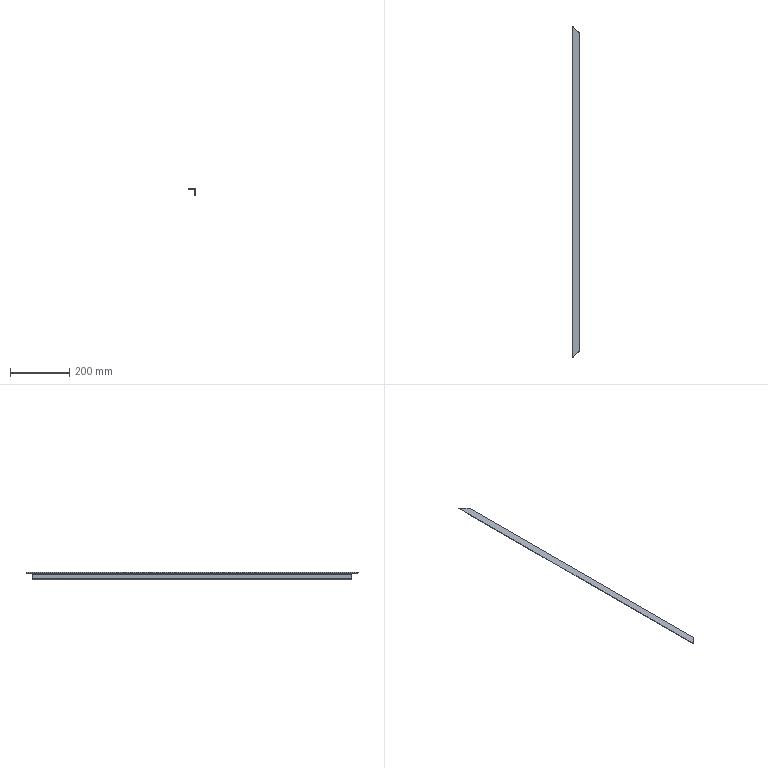Part | STEP file | Guide wheel mechanism revised.sldasm-Part-16 | 1 solid | 9 faces | box 25 x 1120 x 25 mm | volume 195019 mm3 | plane 6 | cylinder 3 | commonest cylinder face diameters 8 x2 7 x1
STEP:
#1=CARTESIAN_POINT('',(-430.,1915.,-505.));
#2=VERTEX_POINT('',#1);
#3=CARTESIAN_POINT('',(-405.,1890.,-505.));
#4=VERTEX_POINT('',#3);
#5=CARTESIAN_POINT('',(117.5,1367.5,-505.));
#6=DIRECTION('',(0.7071,-0.7071,0.));
#7=VECTOR('',#6,1000.);
#8=LINE('',#5,#7);
#9=EDGE_CURVE('',#2,#4,#8,.T.);
#10=ORIENTED_EDGE('',*,*,#9,.F.);
#11=CARTESIAN_POINT('',(-430.,795.,-505.));
#12=VERTEX_POINT('',#11);
#13=CARTESIAN_POINT('',(-430.,820.,-505.));
#14=DIRECTION('',(0.,1.,0.));
#15=VECTOR('',#14,1000.);
#16=LINE('',#13,#15);
#17=EDGE_CURVE('',#12,#2,#16,.T.);
#18=ORIENTED_EDGE('',*,*,#17,.F.);
#19=CARTESIAN_POINT('',(-405.,820.,-505.));
#20=VERTEX_POINT('',#19);
#21=CARTESIAN_POINT('',(-417.5,807.5,-505.));
#22=DIRECTION('',(-0.7071,-0.7071,0.));
#23=VECTOR('',#22,1000.);
#24=LINE('',#21,#23);
#25=EDGE_CURVE('',#20,#12,#24,.T.);
#26=ORIENTED_EDGE('',*,*,#25,.F.);
#27=CARTESIAN_POINT('',(-405.,820.,-505.));
#28=DIRECTION('',(0.,1.,0.));
#29=VECTOR('',#28,1000.);
#30=LINE('',#27,#29);
#31=EDGE_CURVE('',#20,#4,#30,.T.);
#32=ORIENTED_EDGE('',*,*,#31,.T.);
#33=EDGE_LOOP('',(#10,#18,#26,#32));
#34=FACE_OUTER_BOUND('',#33,.T.);
#35=CARTESIAN_POINT('',(-430.,820.,-505.));
#36=DIRECTION('',(0.,0.,-1.));
#37=DIRECTION('',(-1.,0.,0.));
#38=AXIS2_PLACEMENT_3D('',#35,#36,#37);
#39=PLANE('',#38);
#40=ADVANCED_FACE('',(#34),#39,.F.);
#41=CARTESIAN_POINT('',(-426.,1911.,-509.));
#42=VERTEX_POINT('',#41);
#43=CARTESIAN_POINT('',(-426.,1911.,-509.));
#44=CARTESIAN_POINT('',(-428.343,1913.343,-509.));
#45=CARTESIAN_POINT('',(-430.,1915.,-507.343));
#46=CARTESIAN_POINT('',(-430.,1915.,-505.));
#47=(BOUNDED_CURVE()B_SPLINE_CURVE(3,(#43,#44,#45,#46),.UNSPECIFIED.,.F.,.F.)B_SPLINE_CURVE_WITH_KNOTS((4,4),(4.712,6.283),.UNSPECIFIED.)CURVE()GEOMETRIC_REPRESENTATION_ITEM()RATIONAL_B_SPLINE_CURVE((1.,0.8047,0.8047,1.))REPRESENTATION_ITEM(''));
#48=EDGE_CURVE('',#42,#2,#47,.T.);
#49=ORIENTED_EDGE('',*,*,#48,.F.);
#50=CARTESIAN_POINT('',(-426.,799.,-509.));
#51=VERTEX_POINT('',#50);
#52=CARTESIAN_POINT('',(-426.,820.,-509.));
#53=DIRECTION('',(0.,1.,0.));
#54=VECTOR('',#53,1000.);
#55=LINE('',#52,#54);
#56=EDGE_CURVE('',#51,#42,#55,.T.);
#57=ORIENTED_EDGE('',*,*,#56,.F.);
#58=CARTESIAN_POINT('',(-430.,795.,-505.));
#59=CARTESIAN_POINT('',(-430.,795.,-507.343));
#60=CARTESIAN_POINT('',(-428.343,796.657,-509.));
#61=CARTESIAN_POINT('',(-426.,799.,-509.));
#62=(BOUNDED_CURVE()B_SPLINE_CURVE(3,(#58,#59,#60,#61),.UNSPECIFIED.,.F.,.T.)B_SPLINE_CURVE_WITH_KNOTS((4,4),(3.142,4.712),.UNSPECIFIED.)CURVE()GEOMETRIC_REPRESENTATION_ITEM()RATIONAL_B_SPLINE_CURVE((1.,0.8047,0.8047,1.))REPRESENTATION_ITEM(''));
#63=EDGE_CURVE('',#12,#51,#62,.T.);
#64=ORIENTED_EDGE('',*,*,#63,.F.);
#65=ORIENTED_EDGE('',*,*,#17,.T.);
#66=EDGE_LOOP('',(#49,#57,#64,#65));
#67=FACE_OUTER_BOUND('',#66,.T.);
#68=CARTESIAN_POINT('',(-426.,820.,-505.));
#69=DIRECTION('',(0.,1.,0.));
#70=DIRECTION('',(-1.,0.,0.));
#71=AXIS2_PLACEMENT_3D('',#68,#69,#70);
#72=CYLINDRICAL_SURFACE('',#71,4.);
#73=ADVANCED_FACE('',(#67),#72,.T.);
#74=CARTESIAN_POINT('',(-412.5,1897.5,-509.));
#75=VERTEX_POINT('',#74);
#76=CARTESIAN_POINT('',(126.25,1358.75,-509.));
#77=DIRECTION('',(-0.7071,0.7071,0.));
#78=VECTOR('',#77,1000.);
#79=LINE('',#76,#78);
#80=EDGE_CURVE('',#75,#42,#79,.T.);
#81=ORIENTED_EDGE('',*,*,#80,.F.);
#82=CARTESIAN_POINT('',(-412.5,812.5,-509.));
#83=VERTEX_POINT('',#82);
#84=CARTESIAN_POINT('',(-412.5,820.,-509.));
#85=DIRECTION('',(0.,1.,0.));
#86=VECTOR('',#85,1000.);
#87=LINE('',#84,#86);
#88=EDGE_CURVE('',#83,#75,#87,.T.);
#89=ORIENTED_EDGE('',*,*,#88,.F.);
#90=CARTESIAN_POINT('',(-408.75,816.25,-509.));
#91=DIRECTION('',(0.7071,0.7071,0.));
#92=VECTOR('',#91,1000.);
#93=LINE('',#90,#92);
#94=EDGE_CURVE('',#51,#83,#93,.T.);
#95=ORIENTED_EDGE('',*,*,#94,.F.);
#96=ORIENTED_EDGE('',*,*,#56,.T.);
#97=EDGE_LOOP('',(#81,#89,#95,#96));
#98=FACE_OUTER_BOUND('',#97,.T.);
#99=CARTESIAN_POINT('',(-412.5,820.,-509.));
#100=DIRECTION('',(0.,0.,1.));
#101=DIRECTION('',(1.,0.,0.));
#102=AXIS2_PLACEMENT_3D('',#99,#100,#101);
#103=PLANE('',#102);
#104=ADVANCED_FACE('',(#98),#103,.F.);
#105=CARTESIAN_POINT('',(-409.,1894.,-512.5));
#106=VERTEX_POINT('',#105);
#107=CARTESIAN_POINT('',(-409.,1894.,-512.5));
#108=CARTESIAN_POINT('',(-409.,1894.,-510.45));
#109=CARTESIAN_POINT('',(-410.45,1895.45,-509.));
#110=CARTESIAN_POINT('',(-412.5,1897.5,-509.));
#111=(BOUNDED_CURVE()B_SPLINE_CURVE(3,(#107,#108,#109,#110),.UNSPECIFIED.,.F.,.F.)B_SPLINE_CURVE_WITH_KNOTS((4,4),(3.142,4.712),.UNSPECIFIED.)CURVE()GEOMETRIC_REPRESENTATION_ITEM()RATIONAL_B_SPLINE_CURVE((1.,0.8047,0.8047,1.))REPRESENTATION_ITEM(''));
#112=EDGE_CURVE('',#106,#75,#111,.T.);
#113=ORIENTED_EDGE('',*,*,#112,.F.);
#114=CARTESIAN_POINT('',(-409.,816.,-512.5));
#115=VERTEX_POINT('',#114);
#116=CARTESIAN_POINT('',(-409.,820.,-512.5));
#117=DIRECTION('',(0.,1.,0.));
#118=VECTOR('',#117,1000.);
#119=LINE('',#116,#118);
#120=EDGE_CURVE('',#115,#106,#119,.T.);
#121=ORIENTED_EDGE('',*,*,#120,.F.);
#122=CARTESIAN_POINT('',(-412.5,812.5,-509.));
#123=CARTESIAN_POINT('',(-410.45,814.55,-509.));
#124=CARTESIAN_POINT('',(-409.,816.,-510.45));
#125=CARTESIAN_POINT('',(-409.,816.,-512.5));
#126=(BOUNDED_CURVE()B_SPLINE_CURVE(3,(#122,#123,#124,#125),.UNSPECIFIED.,.F.,.F.)B_SPLINE_CURVE_WITH_KNOTS((4,4),(4.712,6.283),.UNSPECIFIED.)CURVE()GEOMETRIC_REPRESENTATION_ITEM()RATIONAL_B_SPLINE_CURVE((1.,0.8047,0.8047,1.))REPRESENTATION_ITEM(''));
#127=EDGE_CURVE('',#83,#115,#126,.T.);
#128=ORIENTED_EDGE('',*,*,#127,.F.);
#129=ORIENTED_EDGE('',*,*,#88,.T.);
#130=EDGE_LOOP('',(#113,#121,#128,#129));
#131=FACE_OUTER_BOUND('',#130,.T.);
#132=CARTESIAN_POINT('',(-412.5,820.,-512.5));
#133=DIRECTION('',(0.,1.,0.));
#134=DIRECTION('',(-1.,0.,0.));
#135=AXIS2_PLACEMENT_3D('',#132,#133,#134);
#136=CYLINDRICAL_SURFACE('',#135,3.5);
#137=ADVANCED_FACE('',(#131),#136,.F.);
#138=CARTESIAN_POINT('',(-409.,1894.,-526.));
#139=VERTEX_POINT('',#138);
#140=CARTESIAN_POINT('',(-409.,1894.,-526.));
#141=DIRECTION('',(0.,0.,1.));
#142=VECTOR('',#141,1000.);
#143=LINE('',#140,#142);
#144=EDGE_CURVE('',#139,#106,#143,.T.);
#145=ORIENTED_EDGE('',*,*,#144,.F.);
#146=CARTESIAN_POINT('',(-409.,816.,-526.));
#147=VERTEX_POINT('',#146);
#148=CARTESIAN_POINT('',(-409.,820.,-526.));
#149=DIRECTION('',(0.,1.,0.));
#150=VECTOR('',#149,1000.);
#151=LINE('',#148,#150);
#152=EDGE_CURVE('',#147,#139,#151,.T.);
#153=ORIENTED_EDGE('',*,*,#152,.F.);
#154=CARTESIAN_POINT('',(-409.,816.,-526.));
#155=DIRECTION('',(0.,0.,-1.));
#156=VECTOR('',#155,1000.);
#157=LINE('',#154,#156);
#158=EDGE_CURVE('',#115,#147,#157,.T.);
#159=ORIENTED_EDGE('',*,*,#158,.F.);
#160=ORIENTED_EDGE('',*,*,#120,.T.);
#161=EDGE_LOOP('',(#145,#153,#159,#160));
#162=FACE_OUTER_BOUND('',#161,.T.);
#163=CARTESIAN_POINT('',(-409.,820.,-526.));
#164=DIRECTION('',(1.,0.,0.));
#165=DIRECTION('',(0.,1.,0.));
#166=AXIS2_PLACEMENT_3D('',#163,#164,#165);
#167=PLANE('',#166);
#168=ADVANCED_FACE('',(#162),#167,.F.);
#169=CARTESIAN_POINT('',(-405.,1890.,-530.));
#170=VERTEX_POINT('',#169);
#171=CARTESIAN_POINT('',(-405.,1890.,-530.));
#172=CARTESIAN_POINT('',(-407.343,1892.343,-530.));
#173=CARTESIAN_POINT('',(-409.,1894.,-528.343));
#174=CARTESIAN_POINT('',(-409.,1894.,-526.));
#175=(BOUNDED_CURVE()B_SPLINE_CURVE(3,(#171,#172,#173,#174),.UNSPECIFIED.,.F.,.F.)B_SPLINE_CURVE_WITH_KNOTS((4,4),(4.712,6.283),.UNSPECIFIED.)CURVE()GEOMETRIC_REPRESENTATION_ITEM()RATIONAL_B_SPLINE_CURVE((1.,0.8047,0.8047,1.))REPRESENTATION_ITEM(''));
#176=EDGE_CURVE('',#170,#139,#175,.T.);
#177=ORIENTED_EDGE('',*,*,#176,.F.);
#178=CARTESIAN_POINT('',(-405.,820.,-530.));
#179=VERTEX_POINT('',#178);
#180=CARTESIAN_POINT('',(-405.,820.,-530.));
#181=DIRECTION('',(0.,1.,0.));
#182=VECTOR('',#181,1000.);
#183=LINE('',#180,#182);
#184=EDGE_CURVE('',#179,#170,#183,.T.);
#185=ORIENTED_EDGE('',*,*,#184,.F.);
#186=CARTESIAN_POINT('',(-409.,816.,-526.));
#187=CARTESIAN_POINT('',(-409.,816.,-528.343));
#188=CARTESIAN_POINT('',(-407.343,817.657,-530.));
#189=CARTESIAN_POINT('',(-405.,820.,-530.));
#190=(BOUNDED_CURVE()B_SPLINE_CURVE(3,(#186,#187,#188,#189),.UNSPECIFIED.,.F.,.F.)B_SPLINE_CURVE_WITH_KNOTS((4,4),(3.142,4.712),.UNSPECIFIED.)CURVE()GEOMETRIC_REPRESENTATION_ITEM()RATIONAL_B_SPLINE_CURVE((1.,0.8047,0.8047,1.))REPRESENTATION_ITEM(''));
#191=EDGE_CURVE('',#147,#179,#190,.T.);
#192=ORIENTED_EDGE('',*,*,#191,.F.);
#193=ORIENTED_EDGE('',*,*,#152,.T.);
#194=EDGE_LOOP('',(#177,#185,#192,#193));
#195=FACE_OUTER_BOUND('',#194,.T.);
#196=CARTESIAN_POINT('',(-405.,820.,-526.));
#197=DIRECTION('',(0.,1.,0.));
#198=DIRECTION('',(-1.,0.,0.));
#199=AXIS2_PLACEMENT_3D('',#196,#197,#198);
#200=CYLINDRICAL_SURFACE('',#199,4.);
#201=ADVANCED_FACE('',(#195),#200,.T.);
#202=CARTESIAN_POINT('',(-405.,1890.,-505.));
#203=DIRECTION('',(0.,0.,-1.));
#204=VECTOR('',#203,1000.);
#205=LINE('',#202,#204);
#206=EDGE_CURVE('',#4,#170,#205,.T.);
#207=ORIENTED_EDGE('',*,*,#206,.F.);
#208=ORIENTED_EDGE('',*,*,#31,.F.);
#209=CARTESIAN_POINT('',(-405.,820.,-505.));
#210=DIRECTION('',(0.,0.,1.));
#211=VECTOR('',#210,1000.);
#212=LINE('',#209,#211);
#213=EDGE_CURVE('',#179,#20,#212,.T.);
#214=ORIENTED_EDGE('',*,*,#213,.F.);
#215=ORIENTED_EDGE('',*,*,#184,.T.);
#216=EDGE_LOOP('',(#207,#208,#214,#215));
#217=FACE_OUTER_BOUND('',#216,.T.);
#218=CARTESIAN_POINT('',(-405.,820.,-505.));
#219=DIRECTION('',(-1.,0.,0.));
#220=DIRECTION('',(0.,-1.,0.));
#221=AXIS2_PLACEMENT_3D('',#218,#219,#220);
#222=PLANE('',#221);
#223=ADVANCED_FACE('',(#217),#222,.F.);
#224=ORIENTED_EDGE('',*,*,#213,.T.);
#225=ORIENTED_EDGE('',*,*,#25,.T.);
#226=ORIENTED_EDGE('',*,*,#63,.T.);
#227=ORIENTED_EDGE('',*,*,#94,.T.);
#228=ORIENTED_EDGE('',*,*,#127,.T.);
#229=ORIENTED_EDGE('',*,*,#158,.T.);
#230=ORIENTED_EDGE('',*,*,#191,.T.);
#231=EDGE_LOOP('',(#224,#225,#226,#227,#228,#229,#230));
#232=FACE_OUTER_BOUND('',#231,.T.);
#233=CARTESIAN_POINT('',(-405.,820.,-505.));
#234=DIRECTION('',(0.7071,-0.7071,0.));
#235=DIRECTION('',(0.7071,0.7071,0.));
#236=AXIS2_PLACEMENT_3D('',#233,#234,#235);
#237=PLANE('',#236);
#238=ADVANCED_FACE('',(#232),#237,.T.);
#239=ORIENTED_EDGE('',*,*,#48,.T.);
#240=ORIENTED_EDGE('',*,*,#9,.T.);
#241=ORIENTED_EDGE('',*,*,#206,.T.);
#242=ORIENTED_EDGE('',*,*,#176,.T.);
#243=ORIENTED_EDGE('',*,*,#144,.T.);
#244=ORIENTED_EDGE('',*,*,#112,.T.);
#245=ORIENTED_EDGE('',*,*,#80,.T.);
#246=EDGE_LOOP('',(#239,#240,#241,#242,#243,#244,#245));
#247=FACE_OUTER_BOUND('',#246,.T.);
#248=CARTESIAN_POINT('',(-405.,1890.,-505.));
#249=DIRECTION('',(0.7071,0.7071,0.));
#250=DIRECTION('',(-0.7071,0.7071,0.));
#251=AXIS2_PLACEMENT_3D('',#248,#249,#250);
#252=PLANE('',#251);
#253=ADVANCED_FACE('',(#247),#252,.T.);
#254=CLOSED_SHELL('',(#40,#73,#104,#137,#168,#201,#223,#238,#253));
#255=MANIFOLD_SOLID_BREP('',#254);
#256=CARTESIAN_POINT('',(0.,0.,0.));
#257=DIRECTION('',(0.,0.,1.));
#258=DIRECTION('',(1.,0.,0.));
#259=AXIS2_PLACEMENT_3D('',#256,#257,#258);
#260=(LENGTH_UNIT()NAMED_UNIT(*)SI_UNIT(.MILLI.,.METRE.));
#261=UNCERTAINTY_MEASURE_WITH_UNIT(LENGTH_MEASURE(0.00001),#260,'','');
#262=(NAMED_UNIT(*)PLANE_ANGLE_UNIT()SI_UNIT($,.RADIAN.));
#263=(NAMED_UNIT(*)SI_UNIT($,.STERADIAN.)SOLID_ANGLE_UNIT());
#264=(GEOMETRIC_REPRESENTATION_CONTEXT(3)GLOBAL_UNCERTAINTY_ASSIGNED_CONTEXT((#261))GLOBAL_UNIT_ASSIGNED_CONTEXT((#260,#262,#263))REPRESENTATION_CONTEXT('',''));
#265=ADVANCED_BREP_SHAPE_REPRESENTATION('',(#255,#259),#264);